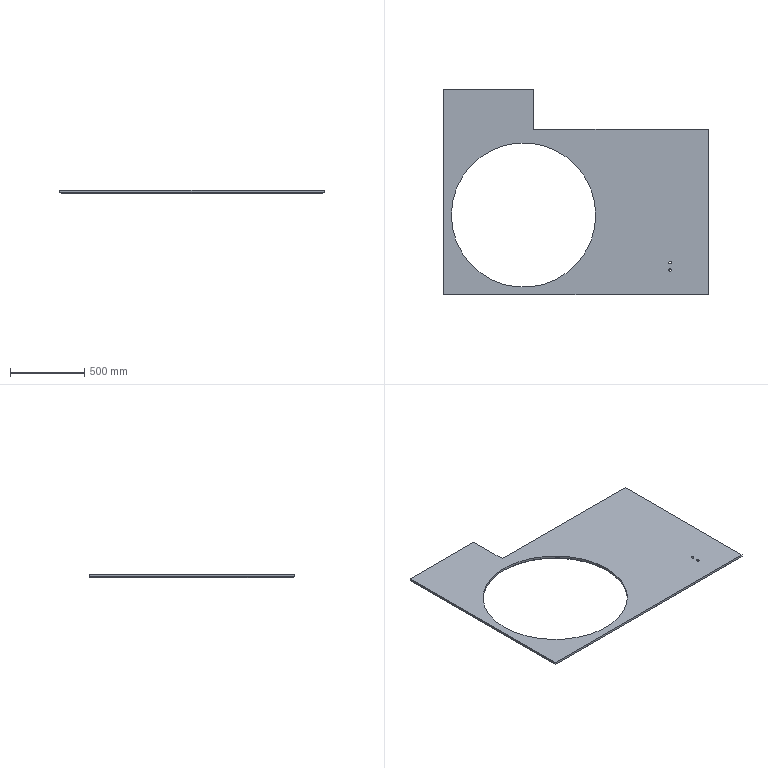Part | SolidWorks | features 3DProfileFeature 1, Chamfer 1, Extrusion 1, HoleWzd 1 | 1 solid | 19 faces | box 1775 x 1380 x 25 mm | volume 34487448 mm3 | plane 11 | cylinder 6 | cone 2 | commonest cylinder face diameters 17.5 x4 970 x2
STEP:
#1=CARTESIAN_POINT('',(1528.75,215.,25.));
#2=VERTEX_POINT('',#1);
#3=CARTESIAN_POINT('',(1511.25,215.,25.));
#4=VERTEX_POINT('',#3);
#5=CARTESIAN_POINT('',(1520.,215.,25.));
#6=DIRECTION('',(0.,0.,-1.));
#7=DIRECTION('',(-1.,0.,0.));
#8=AXIS2_PLACEMENT_3D('',#5,#6,#7);
#9=CIRCLE('',#8,8.75);
#10=EDGE_CURVE('',#2,#4,#9,.T.);
#11=ORIENTED_EDGE('',*,*,#10,.F.);
#12=CARTESIAN_POINT('',(1528.75,215.,0.));
#13=VERTEX_POINT('',#12);
#14=CARTESIAN_POINT('',(1528.75,215.,0.));
#15=DIRECTION('',(0.,0.,-1.));
#16=VECTOR('',#15,1000.);
#17=LINE('',#14,#16);
#18=EDGE_CURVE('',#2,#13,#17,.T.);
#19=ORIENTED_EDGE('',*,*,#18,.T.);
#20=CARTESIAN_POINT('',(1511.25,215.,0.));
#21=VERTEX_POINT('',#20);
#22=CARTESIAN_POINT('',(1520.,215.,0.));
#23=DIRECTION('',(0.,0.,-1.));
#24=DIRECTION('',(-1.,0.,0.));
#25=AXIS2_PLACEMENT_3D('',#22,#23,#24);
#26=CIRCLE('',#25,8.75);
#27=EDGE_CURVE('',#13,#21,#26,.T.);
#28=ORIENTED_EDGE('',*,*,#27,.T.);
#29=CARTESIAN_POINT('',(1511.25,215.,0.));
#30=DIRECTION('',(0.,0.,-1.));
#31=VECTOR('',#30,1000.);
#32=LINE('',#29,#31);
#33=EDGE_CURVE('',#4,#21,#32,.T.);
#34=ORIENTED_EDGE('',*,*,#33,.F.);
#35=EDGE_LOOP('',(#11,#19,#28,#34));
#36=FACE_OUTER_BOUND('',#35,.T.);
#37=CARTESIAN_POINT('',(1520.,215.,0.));
#38=DIRECTION('',(0.,0.,-1.));
#39=DIRECTION('',(-1.,0.,0.));
#40=AXIS2_PLACEMENT_3D('',#37,#38,#39);
#41=CYLINDRICAL_SURFACE('',#40,8.75);
#42=ADVANCED_FACE('',(#36),#41,.F.);
#43=CARTESIAN_POINT('',(1528.75,165.,25.));
#44=VERTEX_POINT('',#43);
#45=CARTESIAN_POINT('',(1511.25,165.,25.));
#46=VERTEX_POINT('',#45);
#47=CARTESIAN_POINT('',(1520.,165.,25.));
#48=DIRECTION('',(0.,0.,-1.));
#49=DIRECTION('',(-1.,0.,0.));
#50=AXIS2_PLACEMENT_3D('',#47,#48,#49);
#51=CIRCLE('',#50,8.75);
#52=EDGE_CURVE('',#44,#46,#51,.T.);
#53=ORIENTED_EDGE('',*,*,#52,.F.);
#54=CARTESIAN_POINT('',(1528.75,165.,0.));
#55=VERTEX_POINT('',#54);
#56=CARTESIAN_POINT('',(1528.75,165.,0.));
#57=DIRECTION('',(0.,0.,-1.));
#58=VECTOR('',#57,1000.);
#59=LINE('',#56,#58);
#60=EDGE_CURVE('',#44,#55,#59,.T.);
#61=ORIENTED_EDGE('',*,*,#60,.T.);
#62=CARTESIAN_POINT('',(1511.25,165.,0.));
#63=VERTEX_POINT('',#62);
#64=CARTESIAN_POINT('',(1520.,165.,0.));
#65=DIRECTION('',(0.,0.,-1.));
#66=DIRECTION('',(-1.,0.,0.));
#67=AXIS2_PLACEMENT_3D('',#64,#65,#66);
#68=CIRCLE('',#67,8.75);
#69=EDGE_CURVE('',#55,#63,#68,.T.);
#70=ORIENTED_EDGE('',*,*,#69,.T.);
#71=CARTESIAN_POINT('',(1511.25,165.,0.));
#72=DIRECTION('',(0.,0.,-1.));
#73=VECTOR('',#72,1000.);
#74=LINE('',#71,#73);
#75=EDGE_CURVE('',#46,#63,#74,.T.);
#76=ORIENTED_EDGE('',*,*,#75,.F.);
#77=EDGE_LOOP('',(#53,#61,#70,#76));
#78=FACE_OUTER_BOUND('',#77,.T.);
#79=CARTESIAN_POINT('',(1520.,165.,0.));
#80=DIRECTION('',(0.,0.,-1.));
#81=DIRECTION('',(-1.,0.,0.));
#82=AXIS2_PLACEMENT_3D('',#79,#80,#81);
#83=CYLINDRICAL_SURFACE('',#82,8.75);
#84=ADVANCED_FACE('',(#78),#83,.F.);
#85=CARTESIAN_POINT('',(1020.,535.,10.));
#86=VERTEX_POINT('',#85);
#87=CARTESIAN_POINT('',(50.,535.,10.));
#88=VERTEX_POINT('',#87);
#89=CARTESIAN_POINT('',(535.,535.,10.));
#90=DIRECTION('',(0.,0.,-1.));
#91=DIRECTION('',(1.,0.,0.));
#92=AXIS2_PLACEMENT_3D('',#89,#90,#91);
#93=CIRCLE('',#92,485.);
#94=EDGE_CURVE('',#86,#88,#93,.T.);
#95=ORIENTED_EDGE('',*,*,#94,.F.);
#96=CARTESIAN_POINT('',(1030.,535.,0.));
#97=VERTEX_POINT('',#96);
#98=CARTESIAN_POINT('',(1030.,535.,0.));
#99=DIRECTION('',(0.7071,0.,-0.7071));
#100=VECTOR('',#99,1000.);
#101=LINE('',#98,#100);
#102=EDGE_CURVE('',#86,#97,#101,.T.);
#103=ORIENTED_EDGE('',*,*,#102,.T.);
#104=CARTESIAN_POINT('',(40.,535.,0.));
#105=VERTEX_POINT('',#104);
#106=CARTESIAN_POINT('',(535.,535.,0.));
#107=DIRECTION('',(0.,0.,1.));
#108=DIRECTION('',(1.,0.,0.));
#109=AXIS2_PLACEMENT_3D('',#106,#107,#108);
#110=CIRCLE('',#109,495.);
#111=EDGE_CURVE('',#105,#97,#110,.T.);
#112=ORIENTED_EDGE('',*,*,#111,.F.);
#113=CARTESIAN_POINT('',(40.,535.,0.));
#114=DIRECTION('',(-0.7071,0.,-0.7071));
#115=VECTOR('',#114,1000.);
#116=LINE('',#113,#115);
#117=EDGE_CURVE('',#88,#105,#116,.T.);
#118=ORIENTED_EDGE('',*,*,#117,.F.);
#119=EDGE_LOOP('',(#95,#103,#112,#118));
#120=FACE_OUTER_BOUND('',#119,.T.);
#121=CARTESIAN_POINT('',(535.,535.,0.));
#122=DIRECTION('',(0.,0.,-1.));
#123=DIRECTION('',(-1.,0.,0.));
#124=AXIS2_PLACEMENT_3D('',#121,#122,#123);
#125=CONICAL_SURFACE('',#124,495.,0.7854);
#126=ADVANCED_FACE('',(#120),#125,.F.);
#127=CARTESIAN_POINT('',(50.,535.,25.));
#128=VERTEX_POINT('',#127);
#129=CARTESIAN_POINT('',(1020.,535.,25.));
#130=VERTEX_POINT('',#129);
#131=CARTESIAN_POINT('',(535.,535.,25.));
#132=DIRECTION('',(0.,0.,1.));
#133=DIRECTION('',(1.,0.,0.));
#134=AXIS2_PLACEMENT_3D('',#131,#132,#133);
#135=CIRCLE('',#134,485.);
#136=EDGE_CURVE('',#128,#130,#135,.T.);
#137=ORIENTED_EDGE('',*,*,#136,.T.);
#138=CARTESIAN_POINT('',(1020.,535.,25.));
#139=DIRECTION('',(0.,0.,-1.));
#140=VECTOR('',#139,1000.);
#141=LINE('',#138,#140);
#142=EDGE_CURVE('',#130,#86,#141,.T.);
#143=ORIENTED_EDGE('',*,*,#142,.T.);
#144=ORIENTED_EDGE('',*,*,#94,.T.);
#145=CARTESIAN_POINT('',(50.,535.,25.));
#146=DIRECTION('',(0.,0.,-1.));
#147=VECTOR('',#146,1000.);
#148=LINE('',#145,#147);
#149=EDGE_CURVE('',#128,#88,#148,.T.);
#150=ORIENTED_EDGE('',*,*,#149,.F.);
#151=EDGE_LOOP('',(#137,#143,#144,#150));
#152=FACE_OUTER_BOUND('',#151,.T.);
#153=CARTESIAN_POINT('',(535.,535.,25.));
#154=DIRECTION('',(0.,0.,-1.));
#155=DIRECTION('',(-1.,0.,0.));
#156=AXIS2_PLACEMENT_3D('',#153,#154,#155);
#157=CYLINDRICAL_SURFACE('',#156,485.);
#158=ADVANCED_FACE('',(#152),#157,.F.);
#159=CARTESIAN_POINT('',(1520.,215.,25.));
#160=DIRECTION('',(0.,0.,-1.));
#161=DIRECTION('',(-1.,0.,0.));
#162=AXIS2_PLACEMENT_3D('',#159,#160,#161);
#163=CIRCLE('',#162,8.75);
#164=EDGE_CURVE('',#4,#2,#163,.T.);
#165=ORIENTED_EDGE('',*,*,#164,.T.);
#166=ORIENTED_EDGE('',*,*,#10,.T.);
#167=EDGE_LOOP('',(#165,#166));
#168=FACE_BOUND('',#167,.T.);
#169=CARTESIAN_POINT('',(1520.,165.,25.));
#170=DIRECTION('',(0.,0.,-1.));
#171=DIRECTION('',(-1.,0.,0.));
#172=AXIS2_PLACEMENT_3D('',#169,#170,#171);
#173=CIRCLE('',#172,8.75);
#174=EDGE_CURVE('',#46,#44,#173,.T.);
#175=ORIENTED_EDGE('',*,*,#174,.T.);
#176=ORIENTED_EDGE('',*,*,#52,.T.);
#177=EDGE_LOOP('',(#175,#176));
#178=FACE_BOUND('',#177,.T.);
#179=CARTESIAN_POINT('',(0.,1380.,25.));
#180=VERTEX_POINT('',#179);
#181=CARTESIAN_POINT('',(0.,0.,25.));
#182=VERTEX_POINT('',#181);
#183=CARTESIAN_POINT('',(0.,1380.,25.));
#184=DIRECTION('',(0.,-1.,0.));
#185=VECTOR('',#184,1000.);
#186=LINE('',#183,#185);
#187=EDGE_CURVE('',#180,#182,#186,.T.);
#188=ORIENTED_EDGE('',*,*,#187,.T.);
#189=CARTESIAN_POINT('',(1775.,0.,25.));
#190=VERTEX_POINT('',#189);
#191=CARTESIAN_POINT('',(0.,0.,25.));
#192=DIRECTION('',(1.,0.,0.));
#193=VECTOR('',#192,1000.);
#194=LINE('',#191,#193);
#195=EDGE_CURVE('',#182,#190,#194,.T.);
#196=ORIENTED_EDGE('',*,*,#195,.T.);
#197=CARTESIAN_POINT('',(1775.,1110.,25.));
#198=VERTEX_POINT('',#197);
#199=CARTESIAN_POINT('',(1775.,0.,25.));
#200=DIRECTION('',(0.,1.,0.));
#201=VECTOR('',#200,1000.);
#202=LINE('',#199,#201);
#203=EDGE_CURVE('',#190,#198,#202,.T.);
#204=ORIENTED_EDGE('',*,*,#203,.T.);
#205=CARTESIAN_POINT('',(605.,1110.,25.));
#206=VERTEX_POINT('',#205);
#207=CARTESIAN_POINT('',(1775.,1110.,25.));
#208=DIRECTION('',(-1.,0.,0.));
#209=VECTOR('',#208,1000.);
#210=LINE('',#207,#209);
#211=EDGE_CURVE('',#198,#206,#210,.T.);
#212=ORIENTED_EDGE('',*,*,#211,.T.);
#213=CARTESIAN_POINT('',(605.,1380.,25.));
#214=VERTEX_POINT('',#213);
#215=CARTESIAN_POINT('',(605.,1110.,25.));
#216=DIRECTION('',(0.,1.,0.));
#217=VECTOR('',#216,1000.);
#218=LINE('',#215,#217);
#219=EDGE_CURVE('',#206,#214,#218,.T.);
#220=ORIENTED_EDGE('',*,*,#219,.T.);
#221=CARTESIAN_POINT('',(605.,1380.,25.));
#222=DIRECTION('',(-1.,0.,0.));
#223=VECTOR('',#222,1000.);
#224=LINE('',#221,#223);
#225=EDGE_CURVE('',#214,#180,#224,.T.);
#226=ORIENTED_EDGE('',*,*,#225,.T.);
#227=EDGE_LOOP('',(#188,#196,#204,#212,#220,#226));
#228=FACE_OUTER_BOUND('',#227,.T.);
#229=ORIENTED_EDGE('',*,*,#136,.F.);
#230=CARTESIAN_POINT('',(535.,535.,25.));
#231=DIRECTION('',(0.,0.,1.));
#232=DIRECTION('',(1.,0.,0.));
#233=AXIS2_PLACEMENT_3D('',#230,#231,#232);
#234=CIRCLE('',#233,485.);
#235=EDGE_CURVE('',#130,#128,#234,.T.);
#236=ORIENTED_EDGE('',*,*,#235,.F.);
#237=EDGE_LOOP('',(#229,#236));
#238=FACE_BOUND('',#237,.T.);
#239=CARTESIAN_POINT('',(0.,0.,25.));
#240=DIRECTION('',(0.,0.,1.));
#241=DIRECTION('',(1.,0.,0.));
#242=AXIS2_PLACEMENT_3D('',#239,#240,#241);
#243=PLANE('',#242);
#244=ADVANCED_FACE('',(#168,#178,#228,#238),#243,.T.);
#245=CARTESIAN_POINT('',(1520.,215.,0.));
#246=DIRECTION('',(0.,0.,-1.));
#247=DIRECTION('',(-1.,0.,0.));
#248=AXIS2_PLACEMENT_3D('',#245,#246,#247);
#249=CIRCLE('',#248,8.75);
#250=EDGE_CURVE('',#21,#13,#249,.T.);
#251=ORIENTED_EDGE('',*,*,#250,.F.);
#252=ORIENTED_EDGE('',*,*,#27,.F.);
#253=EDGE_LOOP('',(#251,#252));
#254=FACE_BOUND('',#253,.T.);
#255=CARTESIAN_POINT('',(1520.,165.,0.));
#256=DIRECTION('',(0.,0.,-1.));
#257=DIRECTION('',(-1.,0.,0.));
#258=AXIS2_PLACEMENT_3D('',#255,#256,#257);
#259=CIRCLE('',#258,8.75);
#260=EDGE_CURVE('',#63,#55,#259,.T.);
#261=ORIENTED_EDGE('',*,*,#260,.F.);
#262=ORIENTED_EDGE('',*,*,#69,.F.);
#263=EDGE_LOOP('',(#261,#262));
#264=FACE_BOUND('',#263,.T.);
#265=ORIENTED_EDGE('',*,*,#111,.T.);
#266=CARTESIAN_POINT('',(535.,535.,0.));
#267=DIRECTION('',(0.,0.,1.));
#268=DIRECTION('',(1.,0.,0.));
#269=AXIS2_PLACEMENT_3D('',#266,#267,#268);
#270=CIRCLE('',#269,495.);
#271=EDGE_CURVE('',#97,#105,#270,.T.);
#272=ORIENTED_EDGE('',*,*,#271,.T.);
#273=EDGE_LOOP('',(#265,#272));
#274=FACE_BOUND('',#273,.T.);
#275=CARTESIAN_POINT('',(1765.,10.,0.));
#276=VERTEX_POINT('',#275);
#277=CARTESIAN_POINT('',(10.,10.,0.));
#278=VERTEX_POINT('',#277);
#279=CARTESIAN_POINT('',(0.,10.,0.));
#280=DIRECTION('',(-1.,0.,0.));
#281=VECTOR('',#280,1000.);
#282=LINE('',#279,#281);
#283=EDGE_CURVE('',#276,#278,#282,.T.);
#284=ORIENTED_EDGE('',*,*,#283,.T.);
#285=CARTESIAN_POINT('',(10.,1380.,0.));
#286=VERTEX_POINT('',#285);
#287=CARTESIAN_POINT('',(10.,0.,0.));
#288=DIRECTION('',(0.,1.,0.));
#289=VECTOR('',#288,1000.);
#290=LINE('',#287,#289);
#291=EDGE_CURVE('',#278,#286,#290,.T.);
#292=ORIENTED_EDGE('',*,*,#291,.T.);
#293=CARTESIAN_POINT('',(605.,1380.,0.));
#294=VERTEX_POINT('',#293);
#295=CARTESIAN_POINT('',(605.,1380.,0.));
#296=DIRECTION('',(-1.,0.,0.));
#297=VECTOR('',#296,1000.);
#298=LINE('',#295,#297);
#299=EDGE_CURVE('',#294,#286,#298,.T.);
#300=ORIENTED_EDGE('',*,*,#299,.F.);
#301=CARTESIAN_POINT('',(605.,1110.,0.));
#302=VERTEX_POINT('',#301);
#303=CARTESIAN_POINT('',(605.,1110.,0.));
#304=DIRECTION('',(0.,1.,0.));
#305=VECTOR('',#304,1000.);
#306=LINE('',#303,#305);
#307=EDGE_CURVE('',#302,#294,#306,.T.);
#308=ORIENTED_EDGE('',*,*,#307,.F.);
#309=CARTESIAN_POINT('',(1765.,1110.,0.));
#310=VERTEX_POINT('',#309);
#311=CARTESIAN_POINT('',(1775.,1110.,0.));
#312=DIRECTION('',(-1.,0.,0.));
#313=VECTOR('',#312,1000.);
#314=LINE('',#311,#313);
#315=EDGE_CURVE('',#310,#302,#314,.T.);
#316=ORIENTED_EDGE('',*,*,#315,.F.);
#317=CARTESIAN_POINT('',(1765.,0.,0.));
#318=DIRECTION('',(0.,-1.,0.));
#319=VECTOR('',#318,1000.);
#320=LINE('',#317,#319);
#321=EDGE_CURVE('',#310,#276,#320,.T.);
#322=ORIENTED_EDGE('',*,*,#321,.T.);
#323=EDGE_LOOP('',(#284,#292,#300,#308,#316,#322));
#324=FACE_OUTER_BOUND('',#323,.T.);
#325=CARTESIAN_POINT('',(0.,0.,0.));
#326=DIRECTION('',(0.,0.,1.));
#327=DIRECTION('',(1.,0.,0.));
#328=AXIS2_PLACEMENT_3D('',#325,#326,#327);
#329=PLANE('',#328);
#330=ADVANCED_FACE('',(#254,#264,#274,#324),#329,.F.);
#331=CARTESIAN_POINT('',(0.,1380.,10.));
#332=VERTEX_POINT('',#331);
#333=CARTESIAN_POINT('',(0.,1380.,25.));
#334=DIRECTION('',(0.,0.,-1.));
#335=VECTOR('',#334,1000.);
#336=LINE('',#333,#335);
#337=EDGE_CURVE('',#180,#332,#336,.T.);
#338=ORIENTED_EDGE('',*,*,#337,.T.);
#339=CARTESIAN_POINT('',(0.,0.,10.));
#340=VERTEX_POINT('',#339);
#341=CARTESIAN_POINT('',(0.,1380.,10.));
#342=DIRECTION('',(0.,-1.,0.));
#343=VECTOR('',#342,1000.);
#344=LINE('',#341,#343);
#345=EDGE_CURVE('',#332,#340,#344,.T.);
#346=ORIENTED_EDGE('',*,*,#345,.T.);
#347=CARTESIAN_POINT('',(0.,0.,25.));
#348=DIRECTION('',(0.,0.,-1.));
#349=VECTOR('',#348,1000.);
#350=LINE('',#347,#349);
#351=EDGE_CURVE('',#182,#340,#350,.T.);
#352=ORIENTED_EDGE('',*,*,#351,.F.);
#353=ORIENTED_EDGE('',*,*,#187,.F.);
#354=EDGE_LOOP('',(#338,#346,#352,#353));
#355=FACE_OUTER_BOUND('',#354,.T.);
#356=CARTESIAN_POINT('',(0.,1380.,25.));
#357=DIRECTION('',(1.,0.,0.));
#358=DIRECTION('',(0.,0.,-1.));
#359=AXIS2_PLACEMENT_3D('',#356,#357,#358);
#360=PLANE('',#359);
#361=ADVANCED_FACE('',(#355),#360,.F.);
#362=ORIENTED_EDGE('',*,*,#351,.T.);
#363=CARTESIAN_POINT('',(1775.,0.,10.));
#364=VERTEX_POINT('',#363);
#365=CARTESIAN_POINT('',(0.,0.,10.));
#366=DIRECTION('',(1.,0.,0.));
#367=VECTOR('',#366,1000.);
#368=LINE('',#365,#367);
#369=EDGE_CURVE('',#340,#364,#368,.T.);
#370=ORIENTED_EDGE('',*,*,#369,.T.);
#371=CARTESIAN_POINT('',(1775.,0.,25.));
#372=DIRECTION('',(0.,0.,-1.));
#373=VECTOR('',#372,1000.);
#374=LINE('',#371,#373);
#375=EDGE_CURVE('',#190,#364,#374,.T.);
#376=ORIENTED_EDGE('',*,*,#375,.F.);
#377=ORIENTED_EDGE('',*,*,#195,.F.);
#378=EDGE_LOOP('',(#362,#370,#376,#377));
#379=FACE_OUTER_BOUND('',#378,.T.);
#380=CARTESIAN_POINT('',(0.,0.,25.));
#381=DIRECTION('',(0.,1.,0.));
#382=DIRECTION('',(0.,0.,1.));
#383=AXIS2_PLACEMENT_3D('',#380,#381,#382);
#384=PLANE('',#383);
#385=ADVANCED_FACE('',(#379),#384,.F.);
#386=ORIENTED_EDGE('',*,*,#375,.T.);
#387=CARTESIAN_POINT('',(1775.,1110.,10.));
#388=VERTEX_POINT('',#387);
#389=CARTESIAN_POINT('',(1775.,0.,10.));
#390=DIRECTION('',(0.,1.,0.));
#391=VECTOR('',#390,1000.);
#392=LINE('',#389,#391);
#393=EDGE_CURVE('',#364,#388,#392,.T.);
#394=ORIENTED_EDGE('',*,*,#393,.T.);
#395=CARTESIAN_POINT('',(1775.,1110.,25.));
#396=DIRECTION('',(0.,0.,-1.));
#397=VECTOR('',#396,1000.);
#398=LINE('',#395,#397);
#399=EDGE_CURVE('',#198,#388,#398,.T.);
#400=ORIENTED_EDGE('',*,*,#399,.F.);
#401=ORIENTED_EDGE('',*,*,#203,.F.);
#402=EDGE_LOOP('',(#386,#394,#400,#401));
#403=FACE_OUTER_BOUND('',#402,.T.);
#404=CARTESIAN_POINT('',(1775.,0.,25.));
#405=DIRECTION('',(-1.,0.,0.));
#406=DIRECTION('',(0.,0.,1.));
#407=AXIS2_PLACEMENT_3D('',#404,#405,#406);
#408=PLANE('',#407);
#409=ADVANCED_FACE('',(#403),#408,.F.);
#410=ORIENTED_EDGE('',*,*,#399,.T.);
#411=CARTESIAN_POINT('',(1775.,1110.,10.));
#412=DIRECTION('',(-0.7071,0.,-0.7071));
#413=VECTOR('',#412,1000.);
#414=LINE('',#411,#413);
#415=EDGE_CURVE('',#388,#310,#414,.T.);
#416=ORIENTED_EDGE('',*,*,#415,.T.);
#417=ORIENTED_EDGE('',*,*,#315,.T.);
#418=CARTESIAN_POINT('',(605.,1110.,25.));
#419=DIRECTION('',(0.,0.,-1.));
#420=VECTOR('',#419,1000.);
#421=LINE('',#418,#420);
#422=EDGE_CURVE('',#206,#302,#421,.T.);
#423=ORIENTED_EDGE('',*,*,#422,.F.);
#424=ORIENTED_EDGE('',*,*,#211,.F.);
#425=EDGE_LOOP('',(#410,#416,#417,#423,#424));
#426=FACE_OUTER_BOUND('',#425,.T.);
#427=CARTESIAN_POINT('',(1775.,1110.,25.));
#428=DIRECTION('',(0.,-1.,0.));
#429=DIRECTION('',(1.,0.,0.));
#430=AXIS2_PLACEMENT_3D('',#427,#428,#429);
#431=PLANE('',#430);
#432=ADVANCED_FACE('',(#426),#431,.F.);
#433=ORIENTED_EDGE('',*,*,#307,.T.);
#434=CARTESIAN_POINT('',(605.,1380.,25.));
#435=DIRECTION('',(0.,0.,-1.));
#436=VECTOR('',#435,1000.);
#437=LINE('',#434,#436);
#438=EDGE_CURVE('',#214,#294,#437,.T.);
#439=ORIENTED_EDGE('',*,*,#438,.F.);
#440=ORIENTED_EDGE('',*,*,#219,.F.);
#441=ORIENTED_EDGE('',*,*,#422,.T.);
#442=EDGE_LOOP('',(#433,#439,#440,#441));
#443=FACE_OUTER_BOUND('',#442,.T.);
#444=CARTESIAN_POINT('',(605.,1110.,25.));
#445=DIRECTION('',(-1.,0.,0.));
#446=DIRECTION('',(0.,0.,1.));
#447=AXIS2_PLACEMENT_3D('',#444,#445,#446);
#448=PLANE('',#447);
#449=ADVANCED_FACE('',(#443),#448,.F.);
#450=ORIENTED_EDGE('',*,*,#299,.T.);
#451=CARTESIAN_POINT('',(0.,1380.,10.));
#452=DIRECTION('',(-0.7071,0.,0.7071));
#453=VECTOR('',#452,1000.);
#454=LINE('',#451,#453);
#455=EDGE_CURVE('',#286,#332,#454,.T.);
#456=ORIENTED_EDGE('',*,*,#455,.T.);
#457=ORIENTED_EDGE('',*,*,#337,.F.);
#458=ORIENTED_EDGE('',*,*,#225,.F.);
#459=ORIENTED_EDGE('',*,*,#438,.T.);
#460=EDGE_LOOP('',(#450,#456,#457,#458,#459));
#461=FACE_OUTER_BOUND('',#460,.T.);
#462=CARTESIAN_POINT('',(605.,1380.,25.));
#463=DIRECTION('',(0.,-1.,0.));
#464=DIRECTION('',(0.,0.,-1.));
#465=AXIS2_PLACEMENT_3D('',#462,#463,#464);
#466=PLANE('',#465);
#467=ADVANCED_FACE('',(#461),#466,.F.);
#468=ORIENTED_EDGE('',*,*,#142,.F.);
#469=ORIENTED_EDGE('',*,*,#235,.T.);
#470=ORIENTED_EDGE('',*,*,#149,.T.);
#471=CARTESIAN_POINT('',(535.,535.,10.));
#472=DIRECTION('',(0.,0.,-1.));
#473=DIRECTION('',(1.,0.,0.));
#474=AXIS2_PLACEMENT_3D('',#471,#472,#473);
#475=CIRCLE('',#474,485.);
#476=EDGE_CURVE('',#88,#86,#475,.T.);
#477=ORIENTED_EDGE('',*,*,#476,.T.);
#478=EDGE_LOOP('',(#468,#469,#470,#477));
#479=FACE_OUTER_BOUND('',#478,.T.);
#480=CARTESIAN_POINT('',(535.,535.,25.));
#481=DIRECTION('',(0.,0.,-1.));
#482=DIRECTION('',(-1.,0.,0.));
#483=AXIS2_PLACEMENT_3D('',#480,#481,#482);
#484=CYLINDRICAL_SURFACE('',#483,485.);
#485=ADVANCED_FACE('',(#479),#484,.F.);
#486=ORIENTED_EDGE('',*,*,#102,.F.);
#487=ORIENTED_EDGE('',*,*,#476,.F.);
#488=ORIENTED_EDGE('',*,*,#117,.T.);
#489=ORIENTED_EDGE('',*,*,#271,.F.);
#490=EDGE_LOOP('',(#486,#487,#488,#489));
#491=FACE_OUTER_BOUND('',#490,.T.);
#492=CARTESIAN_POINT('',(535.,535.,0.));
#493=DIRECTION('',(0.,0.,-1.));
#494=DIRECTION('',(-1.,0.,0.));
#495=AXIS2_PLACEMENT_3D('',#492,#493,#494);
#496=CONICAL_SURFACE('',#495,495.,0.7854);
#497=ADVANCED_FACE('',(#491),#496,.F.);
#498=ORIENTED_EDGE('',*,*,#415,.F.);
#499=ORIENTED_EDGE('',*,*,#393,.F.);
#500=CARTESIAN_POINT('',(1183.333,591.667,-581.667));
#501=DIRECTION('',(0.5774,-0.5774,0.5774));
#502=VECTOR('',#501,1000.);
#503=LINE('',#500,#502);
#504=EDGE_CURVE('',#276,#364,#503,.T.);
#505=ORIENTED_EDGE('',*,*,#504,.F.);
#506=ORIENTED_EDGE('',*,*,#321,.F.);
#507=EDGE_LOOP('',(#498,#499,#505,#506));
#508=FACE_OUTER_BOUND('',#507,.T.);
#509=CARTESIAN_POINT('',(1775.,0.,10.));
#510=DIRECTION('',(-0.7071,0.,0.7071));
#511=DIRECTION('',(0.,1.,0.));
#512=AXIS2_PLACEMENT_3D('',#509,#510,#511);
#513=PLANE('',#512);
#514=ADVANCED_FACE('',(#508),#513,.F.);
#515=ORIENTED_EDGE('',*,*,#504,.T.);
#516=ORIENTED_EDGE('',*,*,#369,.F.);
#517=CARTESIAN_POINT('',(0.,0.,10.));
#518=DIRECTION('',(-0.5774,-0.5774,0.5774));
#519=VECTOR('',#518,1000.);
#520=LINE('',#517,#519);
#521=EDGE_CURVE('',#278,#340,#520,.T.);
#522=ORIENTED_EDGE('',*,*,#521,.F.);
#523=ORIENTED_EDGE('',*,*,#283,.F.);
#524=EDGE_LOOP('',(#515,#516,#522,#523));
#525=FACE_OUTER_BOUND('',#524,.T.);
#526=CARTESIAN_POINT('',(0.,0.,10.));
#527=DIRECTION('',(0.,0.7071,0.7071));
#528=DIRECTION('',(1.,0.,0.));
#529=AXIS2_PLACEMENT_3D('',#526,#527,#528);
#530=PLANE('',#529);
#531=ADVANCED_FACE('',(#525),#530,.F.);
#532=ORIENTED_EDGE('',*,*,#455,.F.);
#533=ORIENTED_EDGE('',*,*,#291,.F.);
#534=ORIENTED_EDGE('',*,*,#521,.T.);
#535=ORIENTED_EDGE('',*,*,#345,.F.);
#536=EDGE_LOOP('',(#532,#533,#534,#535));
#537=FACE_OUTER_BOUND('',#536,.T.);
#538=CARTESIAN_POINT('',(0.,1380.,10.));
#539=DIRECTION('',(0.7071,0.,0.7071));
#540=DIRECTION('',(0.,-1.,0.));
#541=AXIS2_PLACEMENT_3D('',#538,#539,#540);
#542=PLANE('',#541);
#543=ADVANCED_FACE('',(#537),#542,.F.);
#544=ORIENTED_EDGE('',*,*,#60,.F.);
#545=ORIENTED_EDGE('',*,*,#174,.F.);
#546=ORIENTED_EDGE('',*,*,#75,.T.);
#547=ORIENTED_EDGE('',*,*,#260,.T.);
#548=EDGE_LOOP('',(#544,#545,#546,#547));
#549=FACE_OUTER_BOUND('',#548,.T.);
#550=CARTESIAN_POINT('',(1520.,165.,0.));
#551=DIRECTION('',(0.,0.,-1.));
#552=DIRECTION('',(-1.,0.,0.));
#553=AXIS2_PLACEMENT_3D('',#550,#551,#552);
#554=CYLINDRICAL_SURFACE('',#553,8.75);
#555=ADVANCED_FACE('',(#549),#554,.F.);
#556=ORIENTED_EDGE('',*,*,#18,.F.);
#557=ORIENTED_EDGE('',*,*,#164,.F.);
#558=ORIENTED_EDGE('',*,*,#33,.T.);
#559=ORIENTED_EDGE('',*,*,#250,.T.);
#560=EDGE_LOOP('',(#556,#557,#558,#559));
#561=FACE_OUTER_BOUND('',#560,.T.);
#562=CARTESIAN_POINT('',(1520.,215.,0.));
#563=DIRECTION('',(0.,0.,-1.));
#564=DIRECTION('',(-1.,0.,0.));
#565=AXIS2_PLACEMENT_3D('',#562,#563,#564);
#566=CYLINDRICAL_SURFACE('',#565,8.75);
#567=ADVANCED_FACE('',(#561),#566,.F.);
#568=CLOSED_SHELL('',(#42,#84,#126,#158,#244,#330,#361,#385,#409,#432,#449,#467,#485,#497,#514,#531,#543,#555,#567));
#569=MANIFOLD_SOLID_BREP('',#568);
#570=CARTESIAN_POINT('',(0.,0.,0.));
#571=DIRECTION('',(0.,0.,1.));
#572=DIRECTION('',(1.,0.,0.));
#573=AXIS2_PLACEMENT_3D('',#570,#571,#572);
#574=(LENGTH_UNIT()NAMED_UNIT(*)SI_UNIT(.MILLI.,.METRE.));
#575=UNCERTAINTY_MEASURE_WITH_UNIT(LENGTH_MEASURE(0.00001),#574,'','');
#576=(NAMED_UNIT(*)PLANE_ANGLE_UNIT()SI_UNIT($,.RADIAN.));
#577=(NAMED_UNIT(*)SI_UNIT($,.STERADIAN.)SOLID_ANGLE_UNIT());
#578=(GEOMETRIC_REPRESENTATION_CONTEXT(3)GLOBAL_UNCERTAINTY_ASSIGNED_CONTEXT((#575))GLOBAL_UNIT_ASSIGNED_CONTEXT((#574,#576,#577))REPRESENTATION_CONTEXT('',''));
#579=ADVANCED_BREP_SHAPE_REPRESENTATION('',(#569,#573),#578);